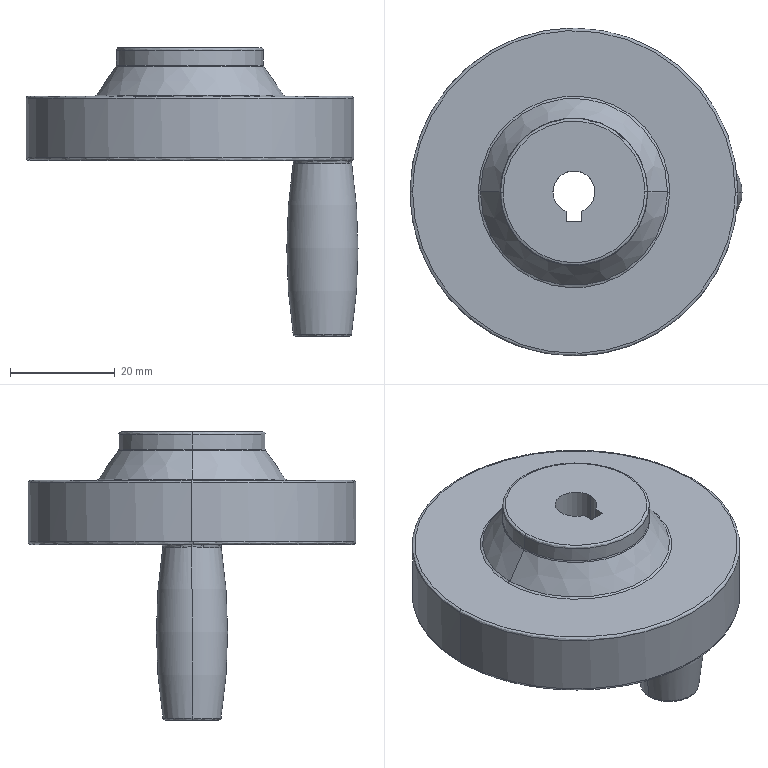Part | SolidWorks | features BaseBody 1 | 1 solid | 47 faces | box 63.283 x 62.5 x 55 mm | volume 41893 mm3 | spline 24 | cylinder 9 | plane 8 | cone 4 | torus 2 | commonest cylinder face diameters 8 x3 28 x2 38.5 x2 62.5 x2